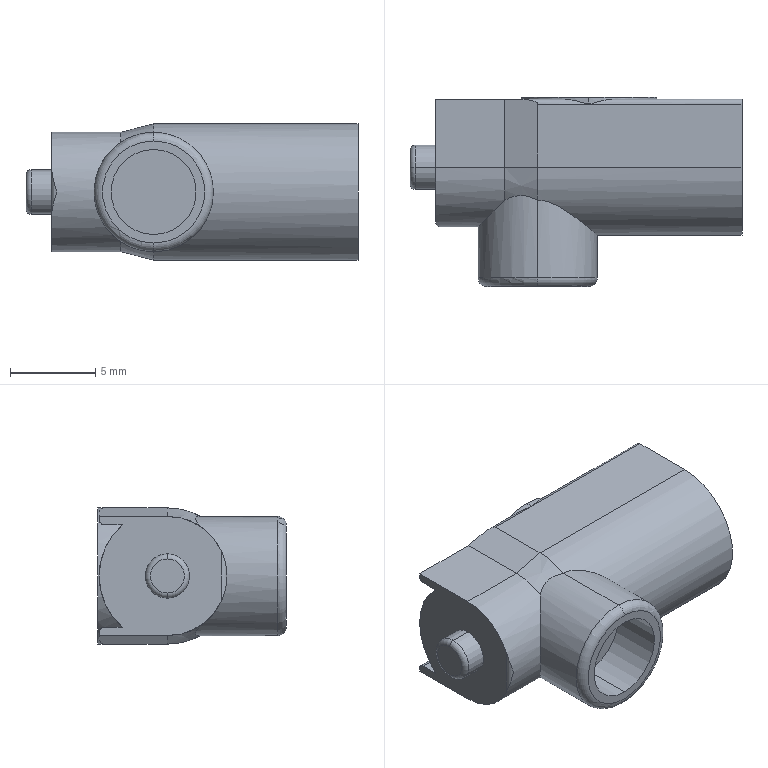Part | SolidWorks | features BaseBody 1 | 1 solid | 47 faces | box 19.5 x 11.1 x 8 mm | volume 1041 mm3 | cylinder 21 | plane 20 | torus 4 | cone 2 | commonest cylinder face diameters 0.6 x9 8 x5 7 x3 2.6 x2 5 x2